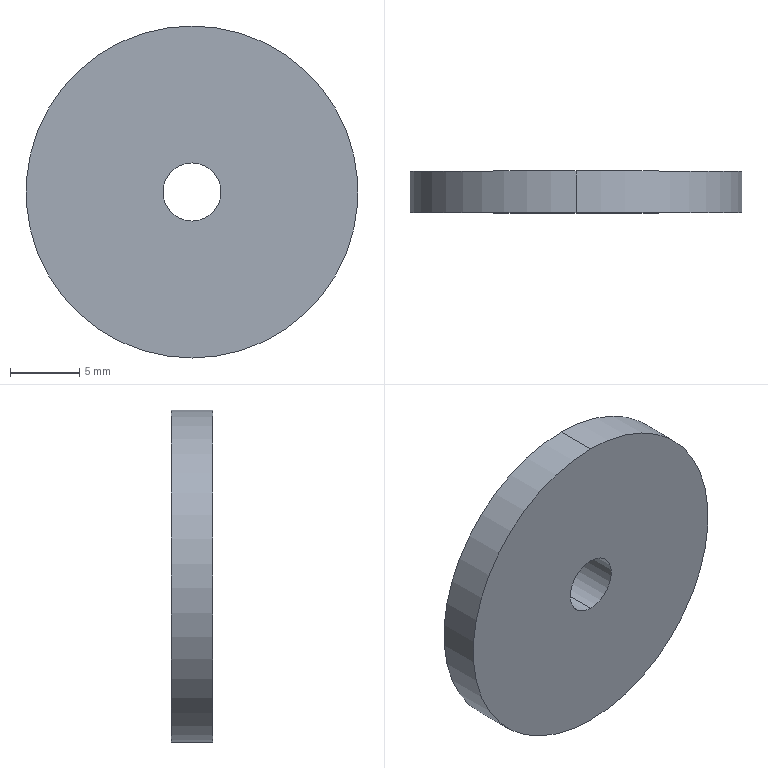Part | SolidWorks | features Extrusion 1 | 1 solid | 6 faces | box 24 x 3 x 24 mm | volume 1316 mm3 | cylinder 4 | plane 2 | commonest cylinder face diameters 4.2 x2 24 x2
STEP:
#1=CARTESIAN_POINT('',(0.,3.,-2.1));
#2=VERTEX_POINT('',#1);
#3=CARTESIAN_POINT('',(0.,3.,2.1));
#4=VERTEX_POINT('',#3);
#5=CARTESIAN_POINT('',(0.,3.,0.));
#6=DIRECTION('',(0.,1.,0.));
#7=DIRECTION('',(0.,0.,1.));
#8=AXIS2_PLACEMENT_3D('',#5,#6,#7);
#9=CIRCLE('',#8,2.1);
#10=EDGE_CURVE('',#2,#4,#9,.T.);
#11=ORIENTED_EDGE('',*,*,#10,.T.);
#12=CARTESIAN_POINT('',(0.,0.,2.1));
#13=VERTEX_POINT('',#12);
#14=CARTESIAN_POINT('',(0.,3.,2.1));
#15=DIRECTION('',(0.,-1.,0.));
#16=VECTOR('',#15,1000.);
#17=LINE('',#14,#16);
#18=EDGE_CURVE('',#4,#13,#17,.T.);
#19=ORIENTED_EDGE('',*,*,#18,.T.);
#20=CARTESIAN_POINT('',(0.,0.,-2.1));
#21=VERTEX_POINT('',#20);
#22=CARTESIAN_POINT('',(0.,0.,0.));
#23=DIRECTION('',(0.,1.,0.));
#24=DIRECTION('',(0.,0.,1.));
#25=AXIS2_PLACEMENT_3D('',#22,#23,#24);
#26=CIRCLE('',#25,2.1);
#27=EDGE_CURVE('',#21,#13,#26,.T.);
#28=ORIENTED_EDGE('',*,*,#27,.F.);
#29=CARTESIAN_POINT('',(0.,3.,-2.1));
#30=DIRECTION('',(0.,-1.,0.));
#31=VECTOR('',#30,1000.);
#32=LINE('',#29,#31);
#33=EDGE_CURVE('',#2,#21,#32,.T.);
#34=ORIENTED_EDGE('',*,*,#33,.F.);
#35=EDGE_LOOP('',(#11,#19,#28,#34));
#36=FACE_OUTER_BOUND('',#35,.T.);
#37=CARTESIAN_POINT('',(0.,3.,0.));
#38=DIRECTION('',(0.,-1.,0.));
#39=DIRECTION('',(0.,0.,-1.));
#40=AXIS2_PLACEMENT_3D('',#37,#38,#39);
#41=CYLINDRICAL_SURFACE('',#40,2.1);
#42=ADVANCED_FACE('',(#36),#41,.F.);
#43=CARTESIAN_POINT('',(0.,3.,12.));
#44=VERTEX_POINT('',#43);
#45=CARTESIAN_POINT('',(0.,3.,-12.));
#46=VERTEX_POINT('',#45);
#47=CARTESIAN_POINT('',(0.,3.,0.));
#48=DIRECTION('',(0.,1.,0.));
#49=DIRECTION('',(0.,0.,1.));
#50=AXIS2_PLACEMENT_3D('',#47,#48,#49);
#51=CIRCLE('',#50,12.);
#52=EDGE_CURVE('',#44,#46,#51,.T.);
#53=ORIENTED_EDGE('',*,*,#52,.F.);
#54=CARTESIAN_POINT('',(0.,0.,12.));
#55=VERTEX_POINT('',#54);
#56=CARTESIAN_POINT('',(0.,3.,12.));
#57=DIRECTION('',(0.,-1.,0.));
#58=VECTOR('',#57,1000.);
#59=LINE('',#56,#58);
#60=EDGE_CURVE('',#44,#55,#59,.T.);
#61=ORIENTED_EDGE('',*,*,#60,.T.);
#62=CARTESIAN_POINT('',(0.,0.,-12.));
#63=VERTEX_POINT('',#62);
#64=CARTESIAN_POINT('',(0.,0.,0.));
#65=DIRECTION('',(0.,1.,0.));
#66=DIRECTION('',(0.,0.,1.));
#67=AXIS2_PLACEMENT_3D('',#64,#65,#66);
#68=CIRCLE('',#67,12.);
#69=EDGE_CURVE('',#55,#63,#68,.T.);
#70=ORIENTED_EDGE('',*,*,#69,.T.);
#71=CARTESIAN_POINT('',(0.,3.,-12.));
#72=DIRECTION('',(0.,-1.,0.));
#73=VECTOR('',#72,1000.);
#74=LINE('',#71,#73);
#75=EDGE_CURVE('',#46,#63,#74,.T.);
#76=ORIENTED_EDGE('',*,*,#75,.F.);
#77=EDGE_LOOP('',(#53,#61,#70,#76));
#78=FACE_OUTER_BOUND('',#77,.T.);
#79=CARTESIAN_POINT('',(0.,3.,0.));
#80=DIRECTION('',(0.,-1.,0.));
#81=DIRECTION('',(0.,0.,-1.));
#82=AXIS2_PLACEMENT_3D('',#79,#80,#81);
#83=CYLINDRICAL_SURFACE('',#82,12.);
#84=ADVANCED_FACE('',(#78),#83,.T.);
#85=CARTESIAN_POINT('',(0.,3.,0.));
#86=DIRECTION('',(0.,1.,0.));
#87=DIRECTION('',(0.,0.,1.));
#88=AXIS2_PLACEMENT_3D('',#85,#86,#87);
#89=CIRCLE('',#88,12.);
#90=EDGE_CURVE('',#46,#44,#89,.T.);
#91=ORIENTED_EDGE('',*,*,#90,.T.);
#92=ORIENTED_EDGE('',*,*,#52,.T.);
#93=EDGE_LOOP('',(#91,#92));
#94=FACE_OUTER_BOUND('',#93,.T.);
#95=ORIENTED_EDGE('',*,*,#10,.F.);
#96=CARTESIAN_POINT('',(0.,3.,0.));
#97=DIRECTION('',(0.,1.,0.));
#98=DIRECTION('',(0.,0.,1.));
#99=AXIS2_PLACEMENT_3D('',#96,#97,#98);
#100=CIRCLE('',#99,2.1);
#101=EDGE_CURVE('',#4,#2,#100,.T.);
#102=ORIENTED_EDGE('',*,*,#101,.F.);
#103=EDGE_LOOP('',(#95,#102));
#104=FACE_BOUND('',#103,.T.);
#105=CARTESIAN_POINT('',(0.,3.,0.));
#106=DIRECTION('',(0.,1.,0.));
#107=DIRECTION('',(0.,0.,1.));
#108=AXIS2_PLACEMENT_3D('',#105,#106,#107);
#109=PLANE('',#108);
#110=ADVANCED_FACE('',(#94,#104),#109,.T.);
#111=CARTESIAN_POINT('',(0.,0.,0.));
#112=DIRECTION('',(0.,1.,0.));
#113=DIRECTION('',(0.,0.,1.));
#114=AXIS2_PLACEMENT_3D('',#111,#112,#113);
#115=CIRCLE('',#114,12.);
#116=EDGE_CURVE('',#63,#55,#115,.T.);
#117=ORIENTED_EDGE('',*,*,#116,.F.);
#118=ORIENTED_EDGE('',*,*,#69,.F.);
#119=EDGE_LOOP('',(#117,#118));
#120=FACE_OUTER_BOUND('',#119,.T.);
#121=ORIENTED_EDGE('',*,*,#27,.T.);
#122=CARTESIAN_POINT('',(0.,0.,0.));
#123=DIRECTION('',(0.,1.,0.));
#124=DIRECTION('',(0.,0.,1.));
#125=AXIS2_PLACEMENT_3D('',#122,#123,#124);
#126=CIRCLE('',#125,2.1);
#127=EDGE_CURVE('',#13,#21,#126,.T.);
#128=ORIENTED_EDGE('',*,*,#127,.T.);
#129=EDGE_LOOP('',(#121,#128));
#130=FACE_BOUND('',#129,.T.);
#131=CARTESIAN_POINT('',(0.,0.,0.));
#132=DIRECTION('',(0.,1.,0.));
#133=DIRECTION('',(0.,0.,1.));
#134=AXIS2_PLACEMENT_3D('',#131,#132,#133);
#135=PLANE('',#134);
#136=ADVANCED_FACE('',(#120,#130),#135,.F.);
#137=ORIENTED_EDGE('',*,*,#60,.F.);
#138=ORIENTED_EDGE('',*,*,#90,.F.);
#139=ORIENTED_EDGE('',*,*,#75,.T.);
#140=ORIENTED_EDGE('',*,*,#116,.T.);
#141=EDGE_LOOP('',(#137,#138,#139,#140));
#142=FACE_OUTER_BOUND('',#141,.T.);
#143=CARTESIAN_POINT('',(0.,3.,0.));
#144=DIRECTION('',(0.,-1.,0.));
#145=DIRECTION('',(0.,0.,-1.));
#146=AXIS2_PLACEMENT_3D('',#143,#144,#145);
#147=CYLINDRICAL_SURFACE('',#146,12.);
#148=ADVANCED_FACE('',(#142),#147,.T.);
#149=ORIENTED_EDGE('',*,*,#18,.F.);
#150=ORIENTED_EDGE('',*,*,#101,.T.);
#151=ORIENTED_EDGE('',*,*,#33,.T.);
#152=ORIENTED_EDGE('',*,*,#127,.F.);
#153=EDGE_LOOP('',(#149,#150,#151,#152));
#154=FACE_OUTER_BOUND('',#153,.T.);
#155=CARTESIAN_POINT('',(0.,3.,0.));
#156=DIRECTION('',(0.,-1.,0.));
#157=DIRECTION('',(0.,0.,-1.));
#158=AXIS2_PLACEMENT_3D('',#155,#156,#157);
#159=CYLINDRICAL_SURFACE('',#158,2.1);
#160=ADVANCED_FACE('',(#154),#159,.F.);
#161=CLOSED_SHELL('',(#42,#84,#110,#136,#148,#160));
#162=MANIFOLD_SOLID_BREP('',#161);
#163=CARTESIAN_POINT('',(0.,0.,0.));
#164=DIRECTION('',(0.,0.,1.));
#165=DIRECTION('',(1.,0.,0.));
#166=AXIS2_PLACEMENT_3D('',#163,#164,#165);
#167=(LENGTH_UNIT()NAMED_UNIT(*)SI_UNIT(.MILLI.,.METRE.));
#168=UNCERTAINTY_MEASURE_WITH_UNIT(LENGTH_MEASURE(0.00001),#167,'','');
#169=(NAMED_UNIT(*)PLANE_ANGLE_UNIT()SI_UNIT($,.RADIAN.));
#170=(NAMED_UNIT(*)SI_UNIT($,.STERADIAN.)SOLID_ANGLE_UNIT());
#171=(GEOMETRIC_REPRESENTATION_CONTEXT(3)GLOBAL_UNCERTAINTY_ASSIGNED_CONTEXT((#168))GLOBAL_UNIT_ASSIGNED_CONTEXT((#167,#169,#170))REPRESENTATION_CONTEXT('',''));
#172=ADVANCED_BREP_SHAPE_REPRESENTATION('',(#162,#166),#171);